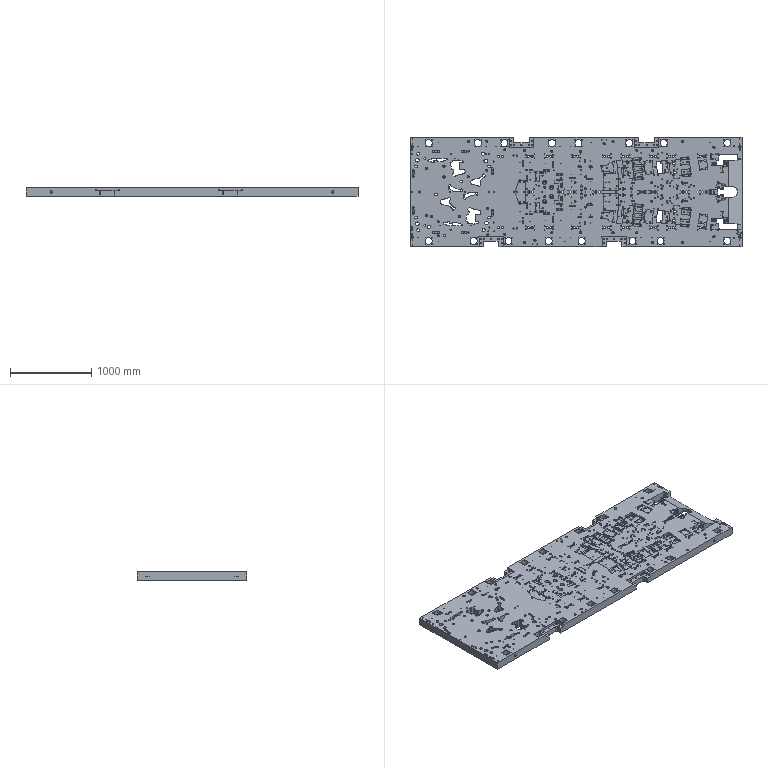Part | NX | features solid 2 | 1 solid | 2704 faces | box 4080 x 1345 x 100 mm | volume 489828052 mm3 | cylinder 1379 | plane 789 | cone 522 | spline 14 | commonest cylinder face diameters 10 x182 10.3 x180 8.5 x170 6.8 x116 20 x96 10.001 x62